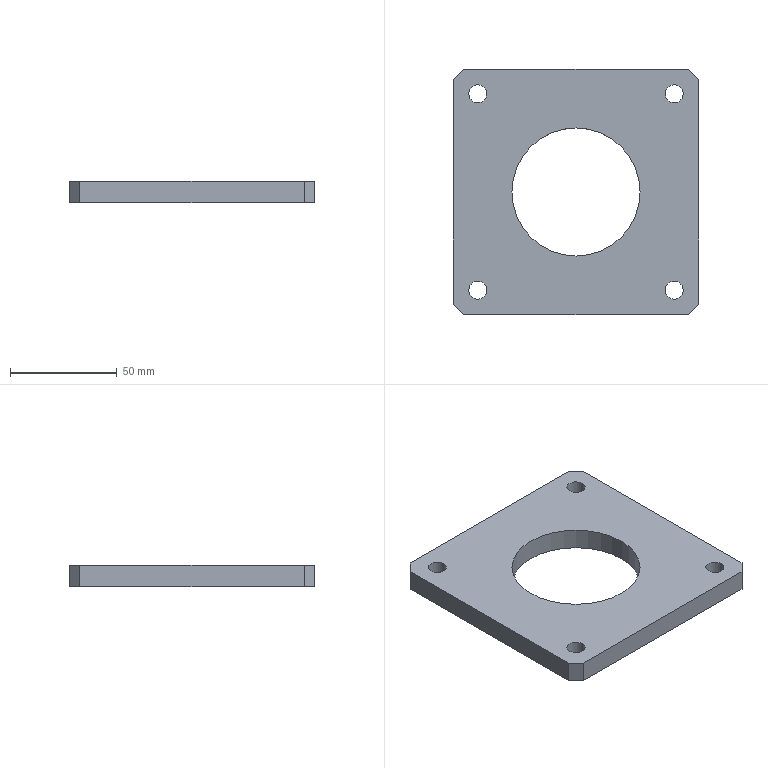Part | STEP file | PN_0033_end plate_default_machined_ | 1 solid | 20 faces | box 115 x 115 x 10 mm | volume 101206 mm3 | cylinder 10 | plane 10 | commonest cylinder face diameters 8.5 x8 60 x2